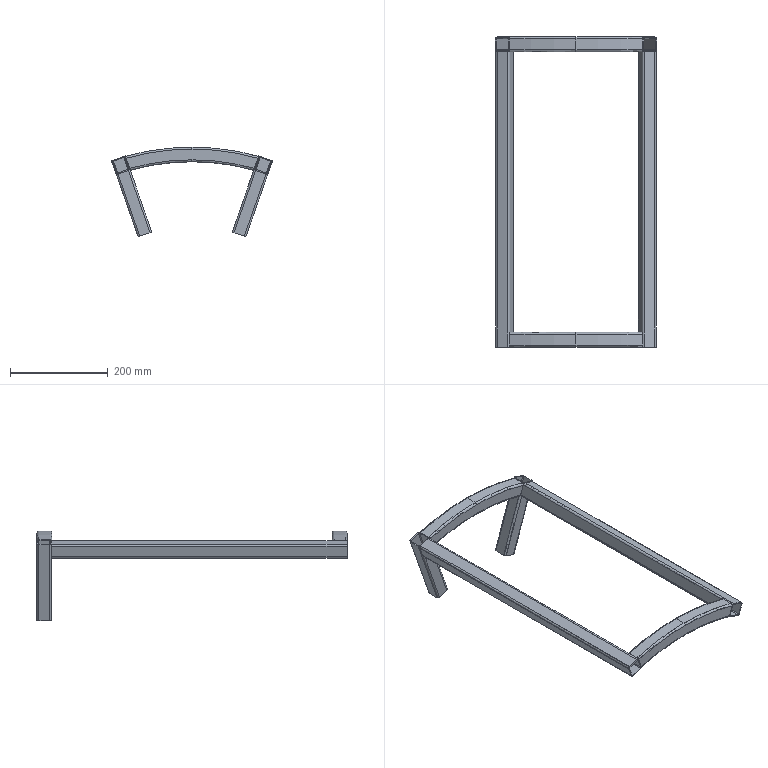Part | SolidWorks | features 3DProfileFeature 1, WeldCornerFeat 1, WeldMemberFeat 1, WeldmentFeature 1 | 6 solids | 136 faces | box 330 x 635 x 183.766 mm | volume 442860 mm3 | cylinder 52 | plane 52 | torus 32 | commonest cylinder face diameters 4 x18 8 x18 940 x4 944 x4 996 x4 1000 x4